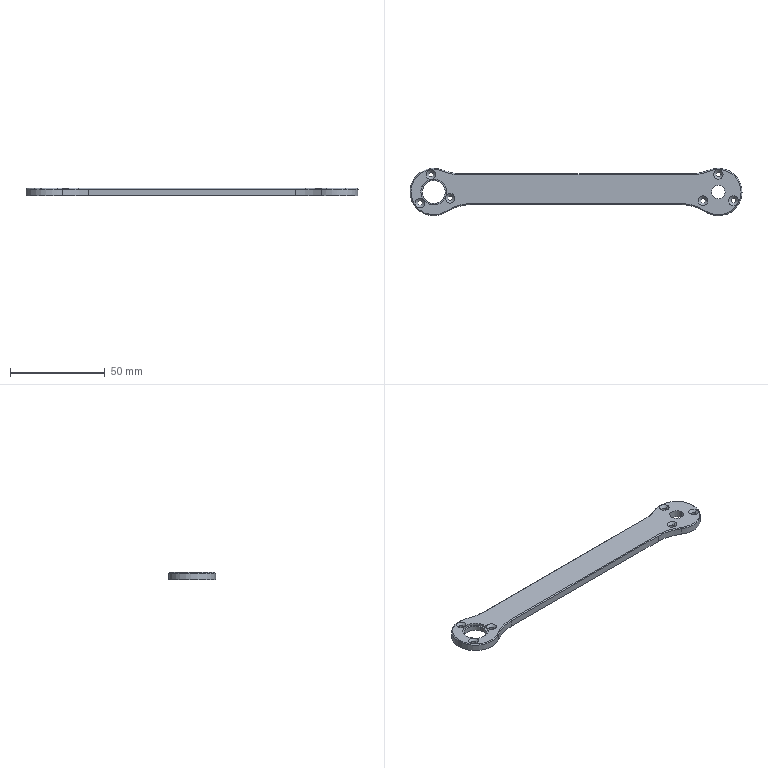Part | NX | features REPLACE_FACE 3, BREP 1 | 1 solid | 57 faces | box 175 x 25 x 4 mm | volume 8666 mm3 | cylinder 29 | cone 16 | plane 12 | commonest cylinder face diameters 2.5 x12 8 x4 50 x4 25 x3 7.1 x2 12 x2